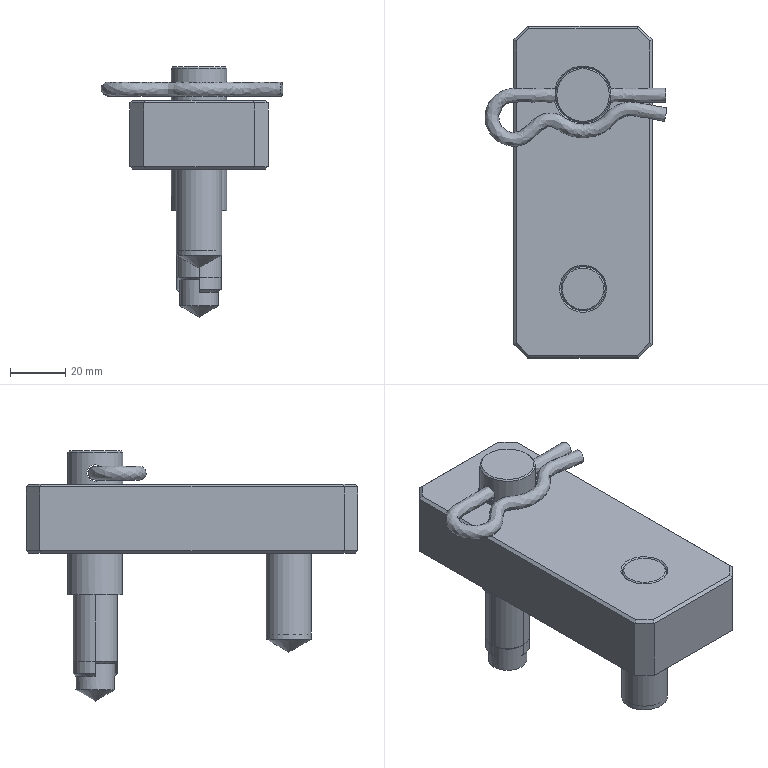Part | STEP file | PH15012004 | 6 solids | 64 faces | box 65.87 x 120 x 90.403 mm | volume 187828 mm3 | plane 40 | cone 12 | cylinder 11 | spline 1 | commonest cylinder face diameters 16 x4 20 x3 6 x1 14 x1 15.947 x1 16.5 x1